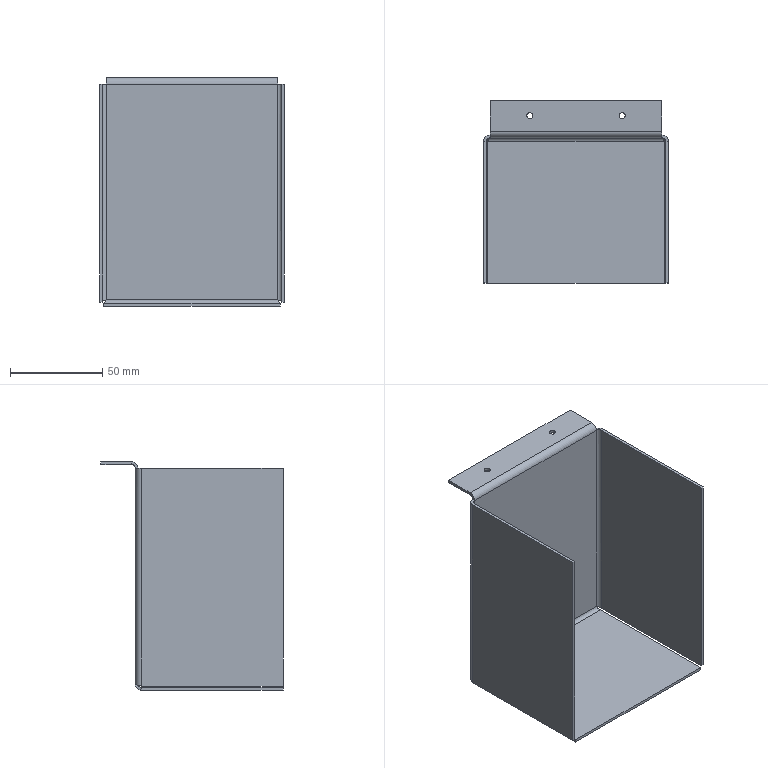Part | NX | features BREP 1 | 1 solid | 42 faces | box 100 x 98.5 x 123.5 mm | volume 59261 mm3 | plane 26 | cylinder 12 | spline 4 | commonest cylinder face diameters 3.3 x4 4 x4 7 x4
STEP:
#1=CARTESIAN_POINT('',(-26.65,10.5,63.5));
#2=VERTEX_POINT('',#1);
#3=CARTESIAN_POINT('',(-26.65,10.5,62.));
#4=VERTEX_POINT('',#3);
#5=CARTESIAN_POINT('',(-26.65,10.5,63.5));
#6=DIRECTION('',(0.,0.,1.));
#7=VECTOR('',#6,1000.);
#8=LINE('',#5,#7);
#9=EDGE_CURVE('',#2,#4,#8,.F.);
#10=ORIENTED_EDGE('',*,*,#9,.T.);
#11=CARTESIAN_POINT('',(-23.35,10.5,62.));
#12=VERTEX_POINT('',#11);
#13=CARTESIAN_POINT('',(-25.,10.5,62.));
#14=DIRECTION('',(0.,0.,1.));
#15=DIRECTION('',(0.,-1.,0.));
#16=AXIS2_PLACEMENT_3D('',#13,#14,#15);
#17=CIRCLE('',#16,1.65);
#18=EDGE_CURVE('',#12,#4,#17,.T.);
#19=ORIENTED_EDGE('',*,*,#18,.F.);
#20=CARTESIAN_POINT('',(-23.35,10.5,63.5));
#21=VERTEX_POINT('',#20);
#22=CARTESIAN_POINT('',(-23.35,10.5,63.5));
#23=DIRECTION('',(0.,0.,1.));
#24=VECTOR('',#23,1000.);
#25=LINE('',#22,#24);
#26=EDGE_CURVE('',#21,#12,#25,.F.);
#27=ORIENTED_EDGE('',*,*,#26,.F.);
#28=CARTESIAN_POINT('',(-25.,10.5,63.5));
#29=DIRECTION('',(0.,0.,1.));
#30=DIRECTION('',(1.,0.,0.));
#31=AXIS2_PLACEMENT_3D('',#28,#29,#30);
#32=CIRCLE('',#31,1.65);
#33=EDGE_CURVE('',#21,#2,#32,.T.);
#34=ORIENTED_EDGE('',*,*,#33,.T.);
#35=EDGE_LOOP('',(#10,#19,#27,#34));
#36=FACE_BOUND('',#35,.T.);
#37=CARTESIAN_POINT('',(-25.,10.5,63.5));
#38=DIRECTION('',(0.,0.,1.));
#39=DIRECTION('',(1.,0.,0.));
#40=AXIS2_PLACEMENT_3D('',#37,#38,#39);
#41=CYLINDRICAL_SURFACE('',#40,1.65);
#42=ADVANCED_FACE('',(#36),#41,.F.);
#43=CARTESIAN_POINT('',(23.35,10.5,63.5));
#44=VERTEX_POINT('',#43);
#45=CARTESIAN_POINT('',(23.35,10.5,62.));
#46=VERTEX_POINT('',#45);
#47=CARTESIAN_POINT('',(23.35,10.5,63.5));
#48=DIRECTION('',(0.,0.,1.));
#49=VECTOR('',#48,1000.);
#50=LINE('',#47,#49);
#51=EDGE_CURVE('',#44,#46,#50,.F.);
#52=ORIENTED_EDGE('',*,*,#51,.T.);
#53=CARTESIAN_POINT('',(26.65,10.5,62.));
#54=VERTEX_POINT('',#53);
#55=CARTESIAN_POINT('',(25.,10.5,62.));
#56=DIRECTION('',(0.,0.,1.));
#57=DIRECTION('',(0.,-1.,0.));
#58=AXIS2_PLACEMENT_3D('',#55,#56,#57);
#59=CIRCLE('',#58,1.65);
#60=EDGE_CURVE('',#54,#46,#59,.T.);
#61=ORIENTED_EDGE('',*,*,#60,.F.);
#62=CARTESIAN_POINT('',(26.65,10.5,63.5));
#63=VERTEX_POINT('',#62);
#64=CARTESIAN_POINT('',(26.65,10.5,63.5));
#65=DIRECTION('',(0.,0.,1.));
#66=VECTOR('',#65,1000.);
#67=LINE('',#64,#66);
#68=EDGE_CURVE('',#63,#54,#67,.F.);
#69=ORIENTED_EDGE('',*,*,#68,.F.);
#70=CARTESIAN_POINT('',(25.,10.5,63.5));
#71=DIRECTION('',(0.,0.,1.));
#72=DIRECTION('',(1.,0.,0.));
#73=AXIS2_PLACEMENT_3D('',#70,#71,#72);
#74=CIRCLE('',#73,1.65);
#75=EDGE_CURVE('',#63,#44,#74,.T.);
#76=ORIENTED_EDGE('',*,*,#75,.T.);
#77=EDGE_LOOP('',(#52,#61,#69,#76));
#78=FACE_BOUND('',#77,.T.);
#79=CARTESIAN_POINT('',(25.,10.5,63.5));
#80=DIRECTION('',(0.,0.,1.));
#81=DIRECTION('',(1.,0.,0.));
#82=AXIS2_PLACEMENT_3D('',#79,#80,#81);
#83=CYLINDRICAL_SURFACE('',#82,1.65);
#84=ADVANCED_FACE('',(#78),#83,.F.);
#85=CARTESIAN_POINT('',(-46.5,18.5,62.));
#86=VERTEX_POINT('',#85);
#87=CARTESIAN_POINT('',(46.5,18.5,62.));
#88=VERTEX_POINT('',#87);
#89=CARTESIAN_POINT('',(0.,18.5,62.));
#90=DIRECTION('',(1.,0.,0.));
#91=VECTOR('',#90,1000.);
#92=LINE('',#89,#91);
#93=EDGE_CURVE('',#86,#88,#92,.T.);
#94=ORIENTED_EDGE('',*,*,#93,.F.);
#95=CARTESIAN_POINT('',(-46.5,18.5,63.5));
#96=VERTEX_POINT('',#95);
#97=CARTESIAN_POINT('',(-46.5,18.5,63.5));
#98=DIRECTION('',(0.,0.,-1.));
#99=VECTOR('',#98,1000.);
#100=LINE('',#97,#99);
#101=EDGE_CURVE('',#96,#86,#100,.T.);
#102=ORIENTED_EDGE('',*,*,#101,.F.);
#103=CARTESIAN_POINT('',(46.5,18.5,63.5));
#104=VERTEX_POINT('',#103);
#105=CARTESIAN_POINT('',(46.5,18.5,63.5));
#106=DIRECTION('',(1.,0.,0.));
#107=VECTOR('',#106,1000.);
#108=LINE('',#105,#107);
#109=EDGE_CURVE('',#96,#104,#108,.T.);
#110=ORIENTED_EDGE('',*,*,#109,.T.);
#111=CARTESIAN_POINT('',(46.5,18.5,63.5));
#112=DIRECTION('',(0.,0.,-1.));
#113=VECTOR('',#112,1000.);
#114=LINE('',#111,#113);
#115=EDGE_CURVE('',#104,#88,#114,.T.);
#116=ORIENTED_EDGE('',*,*,#115,.T.);
#117=EDGE_LOOP('',(#94,#102,#110,#116));
#118=FACE_BOUND('',#117,.T.);
#119=CARTESIAN_POINT('',(46.5,18.5,63.5));
#120=DIRECTION('',(0.,1.,0.));
#121=DIRECTION('',(0.,0.,1.));
#122=AXIS2_PLACEMENT_3D('',#119,#120,#121);
#123=PLANE('',#122);
#124=ADVANCED_FACE('',(#118),#123,.T.);
#125=CARTESIAN_POINT('',(-46.5,2.,62.));
#126=VERTEX_POINT('',#125);
#127=CARTESIAN_POINT('',(46.5,2.,62.));
#128=VERTEX_POINT('',#127);
#129=CARTESIAN_POINT('',(-46.5,2.,62.));
#130=DIRECTION('',(1.,0.,0.));
#131=VECTOR('',#130,1000.);
#132=LINE('',#129,#131);
#133=EDGE_CURVE('',#126,#128,#132,.T.);
#134=ORIENTED_EDGE('',*,*,#133,.F.);
#135=CARTESIAN_POINT('',(-46.5,0.,62.));
#136=DIRECTION('',(0.,1.,0.));
#137=VECTOR('',#136,1000.);
#138=LINE('',#135,#137);
#139=EDGE_CURVE('',#126,#86,#138,.T.);
#140=ORIENTED_EDGE('',*,*,#139,.T.);
#141=ORIENTED_EDGE('',*,*,#93,.T.);
#142=CARTESIAN_POINT('',(46.5,0.,62.));
#143=DIRECTION('',(0.,-1.,0.));
#144=VECTOR('',#143,1000.);
#145=LINE('',#142,#144);
#146=EDGE_CURVE('',#88,#128,#145,.T.);
#147=ORIENTED_EDGE('',*,*,#146,.T.);
#148=EDGE_LOOP('',(#134,#140,#141,#147));
#149=FACE_BOUND('',#148,.T.);
#150=ORIENTED_EDGE('',*,*,#60,.T.);
#151=CARTESIAN_POINT('',(25.,10.5,62.));
#152=DIRECTION('',(0.,0.,1.));
#153=DIRECTION('',(0.,-1.,0.));
#154=AXIS2_PLACEMENT_3D('',#151,#152,#153);
#155=CIRCLE('',#154,1.65);
#156=EDGE_CURVE('',#46,#54,#155,.T.);
#157=ORIENTED_EDGE('',*,*,#156,.T.);
#158=EDGE_LOOP('',(#150,#157));
#159=FACE_BOUND('',#158,.T.);
#160=ORIENTED_EDGE('',*,*,#18,.T.);
#161=CARTESIAN_POINT('',(-25.,10.5,62.));
#162=DIRECTION('',(0.,0.,1.));
#163=DIRECTION('',(0.,-1.,0.));
#164=AXIS2_PLACEMENT_3D('',#161,#162,#163);
#165=CIRCLE('',#164,1.65);
#166=EDGE_CURVE('',#4,#12,#165,.T.);
#167=ORIENTED_EDGE('',*,*,#166,.T.);
#168=EDGE_LOOP('',(#160,#167));
#169=FACE_BOUND('',#168,.T.);
#170=CARTESIAN_POINT('',(0.,0.,62.));
#171=DIRECTION('',(0.,0.,1.));
#172=DIRECTION('',(0.,-1.,0.));
#173=AXIS2_PLACEMENT_3D('',#170,#171,#172);
#174=PLANE('',#173);
#175=ADVANCED_FACE('',(#149,#159,#169),#174,.F.);
#176=CARTESIAN_POINT('',(-46.5,2.,63.5));
#177=VERTEX_POINT('',#176);
#178=CARTESIAN_POINT('',(-46.5,18.5,63.5));
#179=DIRECTION('',(0.,1.,0.));
#180=VECTOR('',#179,1000.);
#181=LINE('',#178,#180);
#182=EDGE_CURVE('',#177,#96,#181,.T.);
#183=ORIENTED_EDGE('',*,*,#182,.F.);
#184=CARTESIAN_POINT('',(46.5,2.,63.5));
#185=VERTEX_POINT('',#184);
#186=CARTESIAN_POINT('',(0.,2.,63.5));
#187=DIRECTION('',(1.,0.,0.));
#188=VECTOR('',#187,1000.);
#189=LINE('',#186,#188);
#190=EDGE_CURVE('',#177,#185,#189,.T.);
#191=ORIENTED_EDGE('',*,*,#190,.T.);
#192=CARTESIAN_POINT('',(46.5,0.,63.5));
#193=DIRECTION('',(0.,-1.,0.));
#194=VECTOR('',#193,1000.);
#195=LINE('',#192,#194);
#196=EDGE_CURVE('',#104,#185,#195,.T.);
#197=ORIENTED_EDGE('',*,*,#196,.F.);
#198=ORIENTED_EDGE('',*,*,#109,.F.);
#199=EDGE_LOOP('',(#183,#191,#197,#198));
#200=FACE_BOUND('',#199,.T.);
#201=ORIENTED_EDGE('',*,*,#75,.F.);
#202=CARTESIAN_POINT('',(25.,10.5,63.5));
#203=DIRECTION('',(0.,0.,1.));
#204=DIRECTION('',(1.,0.,0.));
#205=AXIS2_PLACEMENT_3D('',#202,#203,#204);
#206=CIRCLE('',#205,1.65);
#207=EDGE_CURVE('',#44,#63,#206,.T.);
#208=ORIENTED_EDGE('',*,*,#207,.F.);
#209=EDGE_LOOP('',(#201,#208));
#210=FACE_BOUND('',#209,.T.);
#211=ORIENTED_EDGE('',*,*,#33,.F.);
#212=CARTESIAN_POINT('',(-25.,10.5,63.5));
#213=DIRECTION('',(0.,0.,1.));
#214=DIRECTION('',(1.,0.,0.));
#215=AXIS2_PLACEMENT_3D('',#212,#213,#214);
#216=CIRCLE('',#215,1.65);
#217=EDGE_CURVE('',#2,#21,#216,.T.);
#218=ORIENTED_EDGE('',*,*,#217,.F.);
#219=EDGE_LOOP('',(#211,#218));
#220=FACE_BOUND('',#219,.T.);
#221=CARTESIAN_POINT('',(0.,0.,63.5));
#222=DIRECTION('',(0.,0.,1.));
#223=DIRECTION('',(0.,-1.,0.));
#224=AXIS2_PLACEMENT_3D('',#221,#222,#223);
#225=PLANE('',#224);
#226=ADVANCED_FACE('',(#200,#210,#220),#225,.T.);
#227=ORIENTED_EDGE('',*,*,#139,.F.);
#228=CARTESIAN_POINT('',(-46.5,2.,63.5));
#229=DIRECTION('',(0.,0.,1.));
#230=VECTOR('',#229,1000.);
#231=LINE('',#228,#230);
#232=EDGE_CURVE('',#126,#177,#231,.T.);
#233=ORIENTED_EDGE('',*,*,#232,.T.);
#234=ORIENTED_EDGE('',*,*,#182,.T.);
#235=ORIENTED_EDGE('',*,*,#101,.T.);
#236=EDGE_LOOP('',(#227,#233,#234,#235));
#237=FACE_BOUND('',#236,.T.);
#238=CARTESIAN_POINT('',(-46.5,18.5,63.5));
#239=DIRECTION('',(-1.,0.,0.));
#240=DIRECTION('',(0.,-1.,0.));
#241=AXIS2_PLACEMENT_3D('',#238,#239,#240);
#242=PLANE('',#241);
#243=ADVANCED_FACE('',(#237),#242,.T.);
#244=ORIENTED_EDGE('',*,*,#196,.T.);
#245=CARTESIAN_POINT('',(46.5,2.,62.));
#246=DIRECTION('',(0.,0.,1.));
#247=VECTOR('',#246,1000.);
#248=LINE('',#245,#247);
#249=EDGE_CURVE('',#128,#185,#248,.T.);
#250=ORIENTED_EDGE('',*,*,#249,.F.);
#251=ORIENTED_EDGE('',*,*,#146,.F.);
#252=ORIENTED_EDGE('',*,*,#115,.F.);
#253=EDGE_LOOP('',(#244,#250,#251,#252));
#254=FACE_BOUND('',#253,.T.);
#255=CARTESIAN_POINT('',(46.5,0.,63.5));
#256=DIRECTION('',(1.,0.,0.));
#257=DIRECTION('',(0.,0.,-1.));
#258=AXIS2_PLACEMENT_3D('',#255,#256,#257);
#259=PLANE('',#258);
#260=ADVANCED_FACE('',(#254),#259,.T.);
#261=CARTESIAN_POINT('',(-46.5,0.,60.));
#262=VERTEX_POINT('',#261);
#263=CARTESIAN_POINT('',(46.5,0.,60.));
#264=VERTEX_POINT('',#263);
#265=CARTESIAN_POINT('',(50.,0.,60.));
#266=DIRECTION('',(1.,0.,0.));
#267=VECTOR('',#266,1000.);
#268=LINE('',#265,#267);
#269=EDGE_CURVE('',#262,#264,#268,.T.);
#270=ORIENTED_EDGE('',*,*,#269,.F.);
#271=CARTESIAN_POINT('',(-46.5,2.,60.));
#272=DIRECTION('',(-1.,0.,0.));
#273=DIRECTION('',(0.,0.,-1.));
#274=AXIS2_PLACEMENT_3D('',#271,#272,#273);
#275=CIRCLE('',#274,2.);
#276=EDGE_CURVE('',#262,#126,#275,.T.);
#277=ORIENTED_EDGE('',*,*,#276,.T.);
#278=ORIENTED_EDGE('',*,*,#133,.T.);
#279=CARTESIAN_POINT('',(46.5,2.,60.));
#280=DIRECTION('',(1.,0.,0.));
#281=DIRECTION('',(0.,0.,-1.));
#282=AXIS2_PLACEMENT_3D('',#279,#280,#281);
#283=CIRCLE('',#282,2.);
#284=EDGE_CURVE('',#128,#264,#283,.T.);
#285=ORIENTED_EDGE('',*,*,#284,.T.);
#286=EDGE_LOOP('',(#270,#277,#278,#285));
#287=FACE_BOUND('',#286,.T.);
#288=CARTESIAN_POINT('',(46.5,2.,60.));
#289=DIRECTION('',(1.,0.,0.));
#290=DIRECTION('',(0.,0.,1.));
#291=AXIS2_PLACEMENT_3D('',#288,#289,#290);
#292=CYLINDRICAL_SURFACE('',#291,2.);
#293=ADVANCED_FACE('',(#287),#292,.F.);
#294=CARTESIAN_POINT('',(-46.5,-1.5,60.));
#295=VERTEX_POINT('',#294);
#296=CARTESIAN_POINT('',(46.5,-1.5,60.));
#297=VERTEX_POINT('',#296);
#298=CARTESIAN_POINT('',(50.,-1.5,60.));
#299=DIRECTION('',(1.,0.,0.));
#300=VECTOR('',#299,1000.);
#301=LINE('',#298,#300);
#302=EDGE_CURVE('',#295,#297,#301,.T.);
#303=ORIENTED_EDGE('',*,*,#302,.T.);
#304=CARTESIAN_POINT('',(46.5,2.,60.));
#305=DIRECTION('',(1.,0.,0.));
#306=DIRECTION('',(0.,0.,-1.));
#307=AXIS2_PLACEMENT_3D('',#304,#305,#306);
#308=CIRCLE('',#307,3.5);
#309=EDGE_CURVE('',#185,#297,#308,.T.);
#310=ORIENTED_EDGE('',*,*,#309,.F.);
#311=ORIENTED_EDGE('',*,*,#190,.F.);
#312=CARTESIAN_POINT('',(-46.5,2.,60.));
#313=DIRECTION('',(-1.,0.,0.));
#314=DIRECTION('',(0.,0.,-1.));
#315=AXIS2_PLACEMENT_3D('',#312,#313,#314);
#316=CIRCLE('',#315,3.5);
#317=EDGE_CURVE('',#295,#177,#316,.T.);
#318=ORIENTED_EDGE('',*,*,#317,.F.);
#319=EDGE_LOOP('',(#303,#310,#311,#318));
#320=FACE_BOUND('',#319,.T.);
#321=CARTESIAN_POINT('',(46.5,2.,60.));
#322=DIRECTION('',(1.,0.,0.));
#323=DIRECTION('',(0.,0.,1.));
#324=AXIS2_PLACEMENT_3D('',#321,#322,#323);
#325=CYLINDRICAL_SURFACE('',#324,3.5);
#326=ADVANCED_FACE('',(#320),#325,.T.);
#327=ORIENTED_EDGE('',*,*,#284,.F.);
#328=ORIENTED_EDGE('',*,*,#249,.T.);
#329=ORIENTED_EDGE('',*,*,#309,.T.);
#330=CARTESIAN_POINT('',(46.5,-1.5,60.));
#331=DIRECTION('',(0.,1.,0.));
#332=VECTOR('',#331,1000.);
#333=LINE('',#330,#332);
#334=EDGE_CURVE('',#297,#264,#333,.T.);
#335=ORIENTED_EDGE('',*,*,#334,.T.);
#336=EDGE_LOOP('',(#327,#328,#329,#335));
#337=FACE_BOUND('',#336,.T.);
#338=CARTESIAN_POINT('',(46.5,2.,60.));
#339=DIRECTION('',(-1.,0.,0.));
#340=DIRECTION('',(0.,0.,1.));
#341=AXIS2_PLACEMENT_3D('',#338,#339,#340);
#342=PLANE('',#341);
#343=ADVANCED_FACE('',(#337),#342,.F.);
#344=ORIENTED_EDGE('',*,*,#232,.F.);
#345=ORIENTED_EDGE('',*,*,#276,.F.);
#346=CARTESIAN_POINT('',(-46.5,-1.5,60.));
#347=DIRECTION('',(0.,1.,0.));
#348=VECTOR('',#347,1000.);
#349=LINE('',#346,#348);
#350=EDGE_CURVE('',#295,#262,#349,.T.);
#351=ORIENTED_EDGE('',*,*,#350,.F.);
#352=ORIENTED_EDGE('',*,*,#317,.T.);
#353=EDGE_LOOP('',(#344,#345,#351,#352));
#354=FACE_BOUND('',#353,.T.);
#355=CARTESIAN_POINT('',(-46.5,2.,60.));
#356=DIRECTION('',(-1.,0.,0.));
#357=DIRECTION('',(0.,0.,1.));
#358=AXIS2_PLACEMENT_3D('',#355,#356,#357);
#359=PLANE('',#358);
#360=ADVANCED_FACE('',(#354),#359,.T.);
#361=CARTESIAN_POINT('',(47.793,-3.5,-58.5));
#362=VERTEX_POINT('',#361);
#363=CARTESIAN_POINT('',(47.793,-80.,-58.5));
#364=VERTEX_POINT('',#363);
#365=CARTESIAN_POINT('',(47.793,-1.5,-58.5));
#366=DIRECTION('',(0.,-1.,0.));
#367=VECTOR('',#366,1000.);
#368=LINE('',#365,#367);
#369=EDGE_CURVE('',#362,#364,#368,.T.);
#370=ORIENTED_EDGE('',*,*,#369,.T.);
#371=CARTESIAN_POINT('',(47.793,-80.,-60.));
#372=VERTEX_POINT('',#371);
#373=CARTESIAN_POINT('',(47.793,-80.,-58.5));
#374=DIRECTION('',(0.,0.,-1.));
#375=VECTOR('',#374,1000.);
#376=LINE('',#373,#375);
#377=EDGE_CURVE('',#364,#372,#376,.T.);
#378=ORIENTED_EDGE('',*,*,#377,.T.);
#379=CARTESIAN_POINT('',(47.793,-3.5,-60.));
#380=VERTEX_POINT('',#379);
#381=CARTESIAN_POINT('',(47.793,0.,-60.));
#382=DIRECTION('',(0.,-1.,0.));
#383=VECTOR('',#382,1000.);
#384=LINE('',#381,#383);
#385=EDGE_CURVE('',#380,#372,#384,.T.);
#386=ORIENTED_EDGE('',*,*,#385,.F.);
#387=CARTESIAN_POINT('',(47.793,-3.5,-58.5));
#388=DIRECTION('',(0.,0.,1.));
#389=VECTOR('',#388,1000.);
#390=LINE('',#387,#389);
#391=EDGE_CURVE('',#380,#362,#390,.T.);
#392=ORIENTED_EDGE('',*,*,#391,.T.);
#393=EDGE_LOOP('',(#370,#378,#386,#392));
#394=FACE_BOUND('',#393,.T.);
#395=CARTESIAN_POINT('',(47.793,-1.5,-58.5));
#396=DIRECTION('',(-1.,0.,0.));
#397=DIRECTION('',(0.,-1.,0.));
#398=AXIS2_PLACEMENT_3D('',#395,#396,#397);
#399=PLANE('',#398);
#400=ADVANCED_FACE('',(#394),#399,.F.);
#401=ORIENTED_EDGE('',*,*,#377,.F.);
#402=CARTESIAN_POINT('',(-47.793,-80.,-58.5));
#403=VERTEX_POINT('',#402);
#404=CARTESIAN_POINT('',(0.,-80.,-58.5));
#405=DIRECTION('',(1.,0.,0.));
#406=VECTOR('',#405,1000.);
#407=LINE('',#404,#406);
#408=EDGE_CURVE('',#403,#364,#407,.T.);
#409=ORIENTED_EDGE('',*,*,#408,.F.);
#410=CARTESIAN_POINT('',(-47.793,-80.,-60.));
#411=VERTEX_POINT('',#410);
#412=CARTESIAN_POINT('',(-47.793,-80.,-60.));
#413=DIRECTION('',(0.,0.,-1.));
#414=VECTOR('',#413,1000.);
#415=LINE('',#412,#414);
#416=EDGE_CURVE('',#403,#411,#415,.T.);
#417=ORIENTED_EDGE('',*,*,#416,.T.);
#418=CARTESIAN_POINT('',(-50.,-80.,-60.));
#419=DIRECTION('',(1.,0.,0.));
#420=VECTOR('',#419,1000.);
#421=LINE('',#418,#420);
#422=EDGE_CURVE('',#411,#372,#421,.T.);
#423=ORIENTED_EDGE('',*,*,#422,.T.);
#424=EDGE_LOOP('',(#401,#409,#417,#423));
#425=FACE_BOUND('',#424,.T.);
#426=CARTESIAN_POINT('',(-50.,-80.,-60.));
#427=DIRECTION('',(0.,-1.,0.));
#428=DIRECTION('',(0.,0.,-1.));
#429=AXIS2_PLACEMENT_3D('',#426,#427,#428);
#430=PLANE('',#429);
#431=ADVANCED_FACE('',(#425),#430,.T.);
#432=ORIENTED_EDGE('',*,*,#369,.F.);
#433=CARTESIAN_POINT('',(-47.793,-3.5,-58.5));
#434=VERTEX_POINT('',#433);
#435=CARTESIAN_POINT('',(-50.,-3.5,-58.5));
#436=DIRECTION('',(1.,0.,0.));
#437=VECTOR('',#436,1000.);
#438=LINE('',#435,#437);
#439=EDGE_CURVE('',#434,#362,#438,.T.);
#440=ORIENTED_EDGE('',*,*,#439,.F.);
#441=CARTESIAN_POINT('',(-47.793,0.,-58.5));
#442=DIRECTION('',(0.,-1.,0.));
#443=VECTOR('',#442,1000.);
#444=LINE('',#441,#443);
#445=EDGE_CURVE('',#434,#403,#444,.T.);
#446=ORIENTED_EDGE('',*,*,#445,.T.);
#447=ORIENTED_EDGE('',*,*,#408,.T.);
#448=EDGE_LOOP('',(#432,#440,#446,#447));
#449=FACE_BOUND('',#448,.T.);
#450=CARTESIAN_POINT('',(0.,0.,-58.5));
#451=DIRECTION('',(0.,0.,1.));
#452=DIRECTION('',(0.,-1.,0.));
#453=AXIS2_PLACEMENT_3D('',#450,#451,#452);
#454=PLANE('',#453);
#455=ADVANCED_FACE('',(#449),#454,.T.);
#456=CARTESIAN_POINT('',(-47.793,-3.5,-60.));
#457=VERTEX_POINT('',#456);
#458=CARTESIAN_POINT('',(-50.,-3.5,-60.));
#459=DIRECTION('',(-1.,0.,0.));
#460=VECTOR('',#459,1000.);
#461=LINE('',#458,#460);
#462=EDGE_CURVE('',#380,#457,#461,.T.);
#463=ORIENTED_EDGE('',*,*,#462,.F.);
#464=ORIENTED_EDGE('',*,*,#385,.T.);
#465=ORIENTED_EDGE('',*,*,#422,.F.);
#466=CARTESIAN_POINT('',(-47.793,-1.5,-60.));
#467=DIRECTION('',(0.,-1.,0.));
#468=VECTOR('',#467,1000.);
#469=LINE('',#466,#468);
#470=EDGE_CURVE('',#457,#411,#469,.T.);
#471=ORIENTED_EDGE('',*,*,#470,.F.);
#472=EDGE_LOOP('',(#463,#464,#465,#471));
#473=FACE_BOUND('',#472,.T.);
#474=CARTESIAN_POINT('',(0.,0.,-60.));
#475=DIRECTION('',(0.,0.,1.));
#476=DIRECTION('',(0.,-1.,0.));
#477=AXIS2_PLACEMENT_3D('',#474,#475,#476);
#478=PLANE('',#477);
#479=ADVANCED_FACE('',(#473),#478,.F.);
#480=ORIENTED_EDGE('',*,*,#416,.F.);
#481=ORIENTED_EDGE('',*,*,#445,.F.);
#482=CARTESIAN_POINT('',(-47.793,-3.5,-58.5));
#483=DIRECTION('',(0.,0.,1.));
#484=VECTOR('',#483,1000.);
#485=LINE('',#482,#484);
#486=EDGE_CURVE('',#457,#434,#485,.T.);
#487=ORIENTED_EDGE('',*,*,#486,.F.);
#488=ORIENTED_EDGE('',*,*,#470,.T.);
#489=EDGE_LOOP('',(#480,#481,#487,#488));
#490=FACE_BOUND('',#489,.T.);
#491=CARTESIAN_POINT('',(-47.793,-1.5,-58.5));
#492=DIRECTION('',(-1.,0.,0.));
#493=DIRECTION('',(0.,-1.,0.));
#494=AXIS2_PLACEMENT_3D('',#491,#492,#493);
#495=PLANE('',#494);
#496=ADVANCED_FACE('',(#490),#495,.T.);
#497=CARTESIAN_POINT('',(46.5,-1.5,-56.5));
#498=VERTEX_POINT('',#497);
#499=CARTESIAN_POINT('',(-46.5,-1.5,-56.5));
#500=VERTEX_POINT('',#499);
#501=CARTESIAN_POINT('',(47.793,-1.5,-56.5));
#502=DIRECTION('',(-1.,0.,0.));
#503=VECTOR('',#502,1000.);
#504=LINE('',#501,#503);
#505=EDGE_CURVE('',#498,#500,#504,.T.);
#506=ORIENTED_EDGE('',*,*,#505,.T.);
#507=CARTESIAN_POINT('',(-46.5,-1.5,-56.5));
#508=CARTESIAN_POINT('',(-46.715,-1.5,-57.024));
#509=CARTESIAN_POINT('',(-47.146,-1.933,-58.067));
#510=CARTESIAN_POINT('',(-47.577,-2.976,-58.5));
#511=CARTESIAN_POINT('',(-47.793,-3.5,-58.5));
#512=B_SPLINE_CURVE_WITH_KNOTS('',3,(#507,#508,#509,#510,#511),.UNSPECIFIED.,.F.,.F.,(4,1,4),(0.,0.5,1.),.UNSPECIFIED.);
#513=EDGE_CURVE('',#500,#434,#512,.T.);
#514=ORIENTED_EDGE('',*,*,#513,.T.);
#515=ORIENTED_EDGE('',*,*,#439,.T.);
#516=CARTESIAN_POINT('',(47.793,-3.5,-58.5));
#517=CARTESIAN_POINT('',(47.577,-2.976,-58.5));
#518=CARTESIAN_POINT('',(47.146,-1.933,-58.067));
#519=CARTESIAN_POINT('',(46.715,-1.5,-57.024));
#520=CARTESIAN_POINT('',(46.5,-1.5,-56.5));
#521=B_SPLINE_CURVE_WITH_KNOTS('',3,(#516,#517,#518,#519,#520),.UNSPECIFIED.,.F.,.F.,(4,1,4),(0.,0.5,1.),.UNSPECIFIED.);
#522=EDGE_CURVE('',#362,#498,#521,.T.);
#523=ORIENTED_EDGE('',*,*,#522,.T.);
#524=EDGE_LOOP('',(#506,#514,#515,#523));
#525=FACE_BOUND('',#524,.T.);
#526=CARTESIAN_POINT('',(47.793,-3.5,-56.5));
#527=DIRECTION('',(1.,0.,0.));
#528=DIRECTION('',(0.,0.,-1.));
#529=AXIS2_PLACEMENT_3D('',#526,#527,#528);
#530=CYLINDRICAL_SURFACE('',#529,2.);
#531=ADVANCED_FACE('',(#525),#530,.F.);
#532=CARTESIAN_POINT('',(46.5,0.,-56.5));
#533=VERTEX_POINT('',#532);
#534=CARTESIAN_POINT('',(-46.5,0.,-56.5));
#535=VERTEX_POINT('',#534);
#536=CARTESIAN_POINT('',(47.793,0.,-56.5));
#537=DIRECTION('',(-1.,0.,0.));
#538=VECTOR('',#537,1000.);
#539=LINE('',#536,#538);
#540=EDGE_CURVE('',#533,#535,#539,.T.);
#541=ORIENTED_EDGE('',*,*,#540,.F.);
#542=CARTESIAN_POINT('',(46.5,0.,-56.5));
#543=CARTESIAN_POINT('',(46.715,0.,-57.416));
#544=CARTESIAN_POINT('',(47.146,-0.7584,-59.242));
#545=CARTESIAN_POINT('',(47.577,-2.584,-60.));
#546=CARTESIAN_POINT('',(47.793,-3.5,-60.));
#547=B_SPLINE_CURVE_WITH_KNOTS('',3,(#542,#543,#544,#545,#546),.UNSPECIFIED.,.F.,.F.,(4,1,4),(0.,0.5,1.),.UNSPECIFIED.);
#548=EDGE_CURVE('',#380,#533,#547,.F.);
#549=ORIENTED_EDGE('',*,*,#548,.F.);
#550=ORIENTED_EDGE('',*,*,#462,.T.);
#551=CARTESIAN_POINT('',(-47.793,-3.5,-60.));
#552=CARTESIAN_POINT('',(-47.577,-2.584,-60.));
#553=CARTESIAN_POINT('',(-47.146,-0.7584,-59.242));
#554=CARTESIAN_POINT('',(-46.715,0.,-57.416));
#555=CARTESIAN_POINT('',(-46.5,0.,-56.5));
#556=B_SPLINE_CURVE_WITH_KNOTS('',3,(#551,#552,#553,#554,#555),.UNSPECIFIED.,.F.,.F.,(4,1,4),(0.,0.5,1.),.UNSPECIFIED.);
#557=EDGE_CURVE('',#535,#457,#556,.F.);
#558=ORIENTED_EDGE('',*,*,#557,.F.);
#559=EDGE_LOOP('',(#541,#549,#550,#558));
#560=FACE_BOUND('',#559,.T.);
#561=CARTESIAN_POINT('',(47.793,-3.5,-56.5));
#562=DIRECTION('',(1.,0.,0.));
#563=DIRECTION('',(0.,0.,-1.));
#564=AXIS2_PLACEMENT_3D('',#561,#562,#563);
#565=CYLINDRICAL_SURFACE('',#564,3.5);
#566=ADVANCED_FACE('',(#560),#565,.T.);
#567=ORIENTED_EDGE('',*,*,#522,.F.);
#568=ORIENTED_EDGE('',*,*,#391,.F.);
#569=ORIENTED_EDGE('',*,*,#548,.T.);
#570=CARTESIAN_POINT('',(46.5,-1.5,-56.5));
#571=DIRECTION('',(0.,1.,0.));
#572=VECTOR('',#571,1000.);
#573=LINE('',#570,#572);
#574=EDGE_CURVE('',#498,#533,#573,.T.);
#575=ORIENTED_EDGE('',*,*,#574,.F.);
#576=EDGE_LOOP('',(#567,#568,#569,#575));
#577=FACE_BOUND('',#576,.T.);
#578=CARTESIAN_POINT('',(47.793,-3.5,-60.015));
#579=CARTESIAN_POINT('',(47.685,-3.04,-60.015));
#580=CARTESIAN_POINT('',(47.577,-2.58,-59.924));
#581=CARTESIAN_POINT('',(47.362,-1.73,-59.571));
#582=CARTESIAN_POINT('',(47.254,-1.34,-59.311));
#583=CARTESIAN_POINT('',(47.039,-0.6892,-58.66));
#584=CARTESIAN_POINT('',(46.931,-0.4286,-58.27));
#585=CARTESIAN_POINT('',(46.715,-0.07649,-57.42));
#586=CARTESIAN_POINT('',(46.608,0.015,-56.96));
#587=CARTESIAN_POINT('',(46.5,0.015,-56.5));
#588=CARTESIAN_POINT('',(47.793,-3.5,-60.));
#589=CARTESIAN_POINT('',(47.685,-3.042,-60.));
#590=CARTESIAN_POINT('',(47.577,-2.584,-59.909));
#591=CARTESIAN_POINT('',(47.362,-1.737,-59.558));
#592=CARTESIAN_POINT('',(47.254,-1.349,-59.299));
#593=CARTESIAN_POINT('',(47.039,-0.7012,-58.651));
#594=CARTESIAN_POINT('',(46.931,-0.4417,-58.263));
#595=CARTESIAN_POINT('',(46.715,-0.0911,-57.416));
#596=CARTESIAN_POINT('',(46.608,0.,-56.958));
#597=CARTESIAN_POINT('',(46.5,0.,-56.5));
#598=CARTESIAN_POINT('',(47.793,-3.5,-58.5));
#599=CARTESIAN_POINT('',(47.685,-3.238,-58.5));
#600=CARTESIAN_POINT('',(47.577,-2.977,-58.448));
#601=CARTESIAN_POINT('',(47.362,-2.493,-58.248));
#602=CARTESIAN_POINT('',(47.254,-2.271,-58.099));
#603=CARTESIAN_POINT('',(47.039,-1.901,-57.729));
#604=CARTESIAN_POINT('',(46.931,-1.752,-57.507));
#605=CARTESIAN_POINT('',(46.715,-1.552,-57.023));
#606=CARTESIAN_POINT('',(46.608,-1.5,-56.762));
#607=CARTESIAN_POINT('',(46.5,-1.5,-56.5));
#608=CARTESIAN_POINT('',(47.793,-3.5,-58.485));
#609=CARTESIAN_POINT('',(47.685,-3.24,-58.485));
#610=CARTESIAN_POINT('',(47.577,-2.98,-58.433));
#611=CARTESIAN_POINT('',(47.362,-2.5,-58.234));
#612=CARTESIAN_POINT('',(47.254,-2.28,-58.087));
#613=CARTESIAN_POINT('',(47.039,-1.913,-57.72));
#614=CARTESIAN_POINT('',(46.931,-1.766,-57.5));
#615=CARTESIAN_POINT('',(46.715,-1.567,-57.02));
#616=CARTESIAN_POINT('',(46.608,-1.515,-56.76));
#617=CARTESIAN_POINT('',(46.5,-1.515,-56.5));
#618=B_SPLINE_SURFACE_WITH_KNOTS('',1,3,((#578,#579,#580,#581,#582,#583,#584,#585,#586,#587),(#588,#589,#590,#591,#592,#593,#594,#595,#596,#597),(#598,#599,#600,#601,#602,#603,#604,#605,#606,#607),(#608,#609,#610,#611,#612,#613,#614,#615,#616,#617)),.RULED_SURF.,.F.,.F.,.F.,(2,1,1,2),(4,2,2,2,4),(-0.01,0.,1.,1.01),(0.,0.25,0.5,0.75,1.),.UNSPECIFIED.);
#619=ADVANCED_FACE('',(#577),#618,.F.);
#620=ORIENTED_EDGE('',*,*,#486,.T.);
#621=ORIENTED_EDGE('',*,*,#513,.F.);
#622=CARTESIAN_POINT('',(-46.5,-1.5,-56.5));
#623=DIRECTION('',(0.,1.,0.));
#624=VECTOR('',#623,1000.);
#625=LINE('',#622,#624);
#626=EDGE_CURVE('',#500,#535,#625,.T.);
#627=ORIENTED_EDGE('',*,*,#626,.T.);
#628=ORIENTED_EDGE('',*,*,#557,.T.);
#629=EDGE_LOOP('',(#620,#621,#627,#628));
#630=FACE_BOUND('',#629,.T.);
#631=CARTESIAN_POINT('',(-46.5,0.015,-56.5));
#632=CARTESIAN_POINT('',(-46.608,0.015,-56.96));
#633=CARTESIAN_POINT('',(-46.715,-0.07649,-57.42));
#634=CARTESIAN_POINT('',(-46.931,-0.4286,-58.27));
#635=CARTESIAN_POINT('',(-47.039,-0.6892,-58.66));
#636=CARTESIAN_POINT('',(-47.254,-1.34,-59.311));
#637=CARTESIAN_POINT('',(-47.362,-1.73,-59.571));
#638=CARTESIAN_POINT('',(-47.577,-2.58,-59.924));
#639=CARTESIAN_POINT('',(-47.685,-3.04,-60.015));
#640=CARTESIAN_POINT('',(-47.793,-3.5,-60.015));
#641=CARTESIAN_POINT('',(-46.5,0.,-56.5));
#642=CARTESIAN_POINT('',(-46.608,0.,-56.958));
#643=CARTESIAN_POINT('',(-46.715,-0.0911,-57.416));
#644=CARTESIAN_POINT('',(-46.931,-0.4417,-58.263));
#645=CARTESIAN_POINT('',(-47.039,-0.7012,-58.651));
#646=CARTESIAN_POINT('',(-47.254,-1.349,-59.299));
#647=CARTESIAN_POINT('',(-47.362,-1.737,-59.558));
#648=CARTESIAN_POINT('',(-47.577,-2.584,-59.909));
#649=CARTESIAN_POINT('',(-47.685,-3.042,-60.));
#650=CARTESIAN_POINT('',(-47.793,-3.5,-60.));
#651=CARTESIAN_POINT('',(-46.5,-1.5,-56.5));
#652=CARTESIAN_POINT('',(-46.608,-1.5,-56.762));
#653=CARTESIAN_POINT('',(-46.715,-1.552,-57.023));
#654=CARTESIAN_POINT('',(-46.931,-1.752,-57.507));
#655=CARTESIAN_POINT('',(-47.039,-1.901,-57.729));
#656=CARTESIAN_POINT('',(-47.254,-2.271,-58.099));
#657=CARTESIAN_POINT('',(-47.362,-2.493,-58.248));
#658=CARTESIAN_POINT('',(-47.577,-2.977,-58.448));
#659=CARTESIAN_POINT('',(-47.685,-3.238,-58.5));
#660=CARTESIAN_POINT('',(-47.793,-3.5,-58.5));
#661=CARTESIAN_POINT('',(-46.5,-1.515,-56.5));
#662=CARTESIAN_POINT('',(-46.608,-1.515,-56.76));
#663=CARTESIAN_POINT('',(-46.715,-1.567,-57.02));
#664=CARTESIAN_POINT('',(-46.931,-1.766,-57.5));
#665=CARTESIAN_POINT('',(-47.039,-1.913,-57.72));
#666=CARTESIAN_POINT('',(-47.254,-2.28,-58.087));
#667=CARTESIAN_POINT('',(-47.362,-2.5,-58.234));
#668=CARTESIAN_POINT('',(-47.577,-2.98,-58.433));
#669=CARTESIAN_POINT('',(-47.685,-3.24,-58.485));
#670=CARTESIAN_POINT('',(-47.793,-3.5,-58.485));
#671=B_SPLINE_SURFACE_WITH_KNOTS('',1,3,((#631,#632,#633,#634,#635,#636,#637,#638,#639,#640),(#641,#642,#643,#644,#645,#646,#647,#648,#649,#650),(#651,#652,#653,#654,#655,#656,#657,#658,#659,#660),(#661,#662,#663,#664,#665,#666,#667,#668,#669,#670)),.RULED_SURF.,.F.,.F.,.F.,(2,1,1,2),(4,2,2,2,4),(-0.01,0.,1.,1.01),(0.,0.25,0.5,0.75,1.),.UNSPECIFIED.);
#672=ADVANCED_FACE('',(#630),#671,.F.);
#673=CARTESIAN_POINT('',(50.,-80.,60.));
#674=VERTEX_POINT('',#673);
#675=CARTESIAN_POINT('',(50.,-3.5,60.));
#676=VERTEX_POINT('',#675);
#677=CARTESIAN_POINT('',(50.,-80.,60.));
#678=DIRECTION('',(0.,1.,0.));
#679=VECTOR('',#678,1000.);
#680=LINE('',#677,#679);
#681=EDGE_CURVE('',#674,#676,#680,.T.);
#682=ORIENTED_EDGE('',*,*,#681,.T.);
#683=CARTESIAN_POINT('',(48.5,-3.5,60.));
#684=VERTEX_POINT('',#683);
#685=CARTESIAN_POINT('',(48.5,-3.5,60.));
#686=DIRECTION('',(1.,0.,0.));
#687=VECTOR('',#686,1000.);
#688=LINE('',#685,#687);
#689=EDGE_CURVE('',#684,#676,#688,.T.);
#690=ORIENTED_EDGE('',*,*,#689,.F.);
#691=CARTESIAN_POINT('',(48.5,-80.,60.));
#692=VERTEX_POINT('',#691);
#693=CARTESIAN_POINT('',(48.5,0.,60.));
#694=DIRECTION('',(0.,1.,0.));
#695=VECTOR('',#694,1000.);
#696=LINE('',#693,#695);
#697=EDGE_CURVE('',#692,#684,#696,.T.);
#698=ORIENTED_EDGE('',*,*,#697,.F.);
#699=CARTESIAN_POINT('',(50.,-80.,60.));
#700=DIRECTION('',(-1.,0.,0.));
#701=VECTOR('',#700,1000.);
#702=LINE('',#699,#701);
#703=EDGE_CURVE('',#674,#692,#702,.T.);
#704=ORIENTED_EDGE('',*,*,#703,.F.);
#705=EDGE_LOOP('',(#682,#690,#698,#704));
#706=FACE_BOUND('',#705,.T.);
#707=CARTESIAN_POINT('',(50.,-80.,60.));
#708=DIRECTION('',(0.,0.,1.));
#709=DIRECTION('',(0.,-1.,0.));
#710=AXIS2_PLACEMENT_3D('',#707,#708,#709);
#711=PLANE('',#710);
#712=ADVANCED_FACE('',(#706),#711,.T.);
#713=CARTESIAN_POINT('',(48.5,-80.,-57.793));
#714=VERTEX_POINT('',#713);
#715=CARTESIAN_POINT('',(48.5,-80.,0.));
#716=DIRECTION('',(0.,0.,1.));
#717=VECTOR('',#716,1000.);
#718=LINE('',#715,#717);
#719=EDGE_CURVE('',#714,#692,#718,.T.);
#720=ORIENTED_EDGE('',*,*,#719,.F.);
#721=CARTESIAN_POINT('',(50.,-80.,-57.793));
#722=VERTEX_POINT('',#721);
#723=CARTESIAN_POINT('',(50.,-80.,-57.793));
#724=DIRECTION('',(1.,0.,0.));
#725=VECTOR('',#724,1000.);
#726=LINE('',#723,#725);
#727=EDGE_CURVE('',#714,#722,#726,.T.);
#728=ORIENTED_EDGE('',*,*,#727,.T.);
#729=CARTESIAN_POINT('',(50.,-80.,-60.));
#730=DIRECTION('',(0.,0.,1.));
#731=VECTOR('',#730,1000.);
#732=LINE('',#729,#731);
#733=EDGE_CURVE('',#722,#674,#732,.T.);
#734=ORIENTED_EDGE('',*,*,#733,.T.);
#735=ORIENTED_EDGE('',*,*,#703,.T.);
#736=EDGE_LOOP('',(#720,#728,#734,#735));
#737=FACE_BOUND('',#736,.T.);
#738=CARTESIAN_POINT('',(50.,-80.,-60.));
#739=DIRECTION('',(0.,-1.,0.));
#740=DIRECTION('',(1.,0.,0.));
#741=AXIS2_PLACEMENT_3D('',#738,#739,#740);
#742=PLANE('',#741);
#743=ADVANCED_FACE('',(#737),#742,.T.);
#744=CARTESIAN_POINT('',(48.5,-3.5,-57.793));
#745=VERTEX_POINT('',#744);
#746=CARTESIAN_POINT('',(48.5,-3.5,-60.));
#747=DIRECTION('',(0.,0.,1.));
#748=VECTOR('',#747,1000.);
#749=LINE('',#746,#748);
#750=EDGE_CURVE('',#745,#684,#749,.T.);
#751=ORIENTED_EDGE('',*,*,#750,.F.);
#752=CARTESIAN_POINT('',(48.5,0.,-57.793));
#753=DIRECTION('',(0.,-1.,0.));
#754=VECTOR('',#753,1000.);
#755=LINE('',#752,#754);
#756=EDGE_CURVE('',#745,#714,#755,.T.);
#757=ORIENTED_EDGE('',*,*,#756,.T.);
#758=ORIENTED_EDGE('',*,*,#719,.T.);
#759=ORIENTED_EDGE('',*,*,#697,.T.);
#760=EDGE_LOOP('',(#751,#757,#758,#759));
#761=FACE_BOUND('',#760,.T.);
#762=CARTESIAN_POINT('',(48.5,0.,0.));
#763=DIRECTION('',(-1.,0.,0.));
#764=DIRECTION('',(0.,-1.,0.));
#765=AXIS2_PLACEMENT_3D('',#762,#763,#764);
#766=PLANE('',#765);
#767=ADVANCED_FACE('',(#761),#766,.T.);
#768=CARTESIAN_POINT('',(50.,-3.5,-57.793));
#769=VERTEX_POINT('',#768);
#770=CARTESIAN_POINT('',(50.,-1.5,-57.793));
#771=DIRECTION('',(0.,-1.,0.));
#772=VECTOR('',#771,1000.);
#773=LINE('',#770,#772);
#774=EDGE_CURVE('',#769,#722,#773,.T.);
#775=ORIENTED_EDGE('',*,*,#774,.F.);
#776=CARTESIAN_POINT('',(50.,-3.5,-60.));
#777=DIRECTION('',(0.,0.,-1.));
#778=VECTOR('',#777,1000.);
#779=LINE('',#776,#778);
#780=EDGE_CURVE('',#676,#769,#779,.T.);
#781=ORIENTED_EDGE('',*,*,#780,.F.);
#782=ORIENTED_EDGE('',*,*,#681,.F.);
#783=ORIENTED_EDGE('',*,*,#733,.F.);
#784=EDGE_LOOP('',(#775,#781,#782,#783));
#785=FACE_BOUND('',#784,.T.);
#786=CARTESIAN_POINT('',(50.,0.,0.));
#787=DIRECTION('',(-1.,0.,0.));
#788=DIRECTION('',(0.,-1.,0.));
#789=AXIS2_PLACEMENT_3D('',#786,#787,#788);
#790=PLANE('',#789);
#791=ADVANCED_FACE('',(#785),#790,.F.);
#792=ORIENTED_EDGE('',*,*,#727,.F.);
#793=ORIENTED_EDGE('',*,*,#756,.F.);
#794=CARTESIAN_POINT('',(48.5,-3.5,-57.793));
#795=DIRECTION('',(-1.,0.,0.));
#796=VECTOR('',#795,1000.);
#797=LINE('',#794,#796);
#798=EDGE_CURVE('',#769,#745,#797,.T.);
#799=ORIENTED_EDGE('',*,*,#798,.F.);
#800=ORIENTED_EDGE('',*,*,#774,.T.);
#801=EDGE_LOOP('',(#792,#793,#799,#800));
#802=FACE_BOUND('',#801,.T.);
#803=CARTESIAN_POINT('',(48.5,-1.5,-57.793));
#804=DIRECTION('',(0.,0.,-1.));
#805=DIRECTION('',(0.,1.,0.));
#806=AXIS2_PLACEMENT_3D('',#803,#804,#805);
#807=PLANE('',#806);
#808=ADVANCED_FACE('',(#802),#807,.T.);
#809=CARTESIAN_POINT('',(46.5,-1.5,60.));
#810=DIRECTION('',(0.,0.,-1.));
#811=VECTOR('',#810,1000.);
#812=LINE('',#809,#811);
#813=EDGE_CURVE('',#297,#498,#812,.T.);
#814=ORIENTED_EDGE('',*,*,#813,.T.);
#815=CARTESIAN_POINT('',(46.5,-1.5,-56.5));
#816=CARTESIAN_POINT('',(47.024,-1.5,-56.715));
#817=CARTESIAN_POINT('',(48.067,-1.933,-57.146));
#818=CARTESIAN_POINT('',(48.5,-2.976,-57.577));
#819=CARTESIAN_POINT('',(48.5,-3.5,-57.793));
#820=B_SPLINE_CURVE_WITH_KNOTS('',3,(#815,#816,#817,#818,#819),.UNSPECIFIED.,.F.,.F.,(4,1,4),(0.,0.5,1.),.UNSPECIFIED.);
#821=EDGE_CURVE('',#498,#745,#820,.T.);
#822=ORIENTED_EDGE('',*,*,#821,.T.);
#823=ORIENTED_EDGE('',*,*,#750,.T.);
#824=CARTESIAN_POINT('',(46.5,-3.5,60.));
#825=DIRECTION('',(0.,0.,1.));
#826=DIRECTION('',(1.,0.,0.));
#827=AXIS2_PLACEMENT_3D('',#824,#825,#826);
#828=CIRCLE('',#827,2.);
#829=EDGE_CURVE('',#684,#297,#828,.T.);
#830=ORIENTED_EDGE('',*,*,#829,.T.);
#831=EDGE_LOOP('',(#814,#822,#823,#830));
#832=FACE_BOUND('',#831,.T.);
#833=CARTESIAN_POINT('',(46.5,-3.5,60.));
#834=DIRECTION('',(0.,0.,1.));
#835=DIRECTION('',(1.,0.,0.));
#836=AXIS2_PLACEMENT_3D('',#833,#834,#835);
#837=CYLINDRICAL_SURFACE('',#836,2.);
#838=ADVANCED_FACE('',(#832),#837,.F.);
#839=CARTESIAN_POINT('',(46.5,0.,60.));
#840=DIRECTION('',(0.,0.,-1.));
#841=VECTOR('',#840,1000.);
#842=LINE('',#839,#841);
#843=EDGE_CURVE('',#264,#533,#842,.T.);
#844=ORIENTED_EDGE('',*,*,#843,.F.);
#845=CARTESIAN_POINT('',(46.5,-3.5,60.));
#846=DIRECTION('',(0.,0.,1.));
#847=DIRECTION('',(1.,0.,0.));
#848=AXIS2_PLACEMENT_3D('',#845,#846,#847);
#849=CIRCLE('',#848,3.5);
#850=EDGE_CURVE('',#676,#264,#849,.T.);
#851=ORIENTED_EDGE('',*,*,#850,.F.);
#852=ORIENTED_EDGE('',*,*,#780,.T.);
#853=CARTESIAN_POINT('',(50.,-3.5,-57.793));
#854=CARTESIAN_POINT('',(50.,-2.584,-57.577));
#855=CARTESIAN_POINT('',(49.242,-0.7584,-57.146));
#856=CARTESIAN_POINT('',(47.416,0.,-56.715));
#857=CARTESIAN_POINT('',(46.5,0.,-56.5));
#858=B_SPLINE_CURVE_WITH_KNOTS('',3,(#853,#854,#855,#856,#857),.UNSPECIFIED.,.F.,.F.,(4,1,4),(0.,0.5,1.),.UNSPECIFIED.);
#859=EDGE_CURVE('',#533,#769,#858,.F.);
#860=ORIENTED_EDGE('',*,*,#859,.F.);
#861=EDGE_LOOP('',(#844,#851,#852,#860));
#862=FACE_BOUND('',#861,.T.);
#863=CARTESIAN_POINT('',(46.5,-3.5,60.));
#864=DIRECTION('',(0.,0.,1.));
#865=DIRECTION('',(1.,0.,0.));
#866=AXIS2_PLACEMENT_3D('',#863,#864,#865);
#867=CYLINDRICAL_SURFACE('',#866,3.5);
#868=ADVANCED_FACE('',(#862),#867,.T.);
#869=ORIENTED_EDGE('',*,*,#829,.F.);
#870=ORIENTED_EDGE('',*,*,#689,.T.);
#871=ORIENTED_EDGE('',*,*,#850,.T.);
#872=ORIENTED_EDGE('',*,*,#334,.F.);
#873=EDGE_LOOP('',(#869,#870,#871,#872));
#874=FACE_BOUND('',#873,.T.);
#875=CARTESIAN_POINT('',(46.5,-3.5,60.));
#876=DIRECTION('',(0.,0.,-1.));
#877=DIRECTION('',(-1.,0.,0.));
#878=AXIS2_PLACEMENT_3D('',#875,#876,#877);
#879=PLANE('',#878);
#880=ADVANCED_FACE('',(#874),#879,.F.);
#881=ORIENTED_EDGE('',*,*,#798,.T.);
#882=ORIENTED_EDGE('',*,*,#821,.F.);
#883=ORIENTED_EDGE('',*,*,#574,.T.);
#884=ORIENTED_EDGE('',*,*,#859,.T.);
#885=EDGE_LOOP('',(#881,#882,#883,#884));
#886=FACE_BOUND('',#885,.T.);
#887=CARTESIAN_POINT('',(46.5,0.015,-56.5));
#888=CARTESIAN_POINT('',(46.96,0.015,-56.608));
#889=CARTESIAN_POINT('',(47.42,-0.07649,-56.715));
#890=CARTESIAN_POINT('',(48.27,-0.4286,-56.931));
#891=CARTESIAN_POINT('',(48.66,-0.6892,-57.039));
#892=CARTESIAN_POINT('',(49.311,-1.34,-57.254));
#893=CARTESIAN_POINT('',(49.571,-1.73,-57.362));
#894=CARTESIAN_POINT('',(49.924,-2.58,-57.577));
#895=CARTESIAN_POINT('',(50.015,-3.04,-57.685));
#896=CARTESIAN_POINT('',(50.015,-3.5,-57.793));
#897=CARTESIAN_POINT('',(46.5,0.,-56.5));
#898=CARTESIAN_POINT('',(46.958,0.,-56.608));
#899=CARTESIAN_POINT('',(47.416,-0.0911,-56.715));
#900=CARTESIAN_POINT('',(48.263,-0.4417,-56.931));
#901=CARTESIAN_POINT('',(48.651,-0.7012,-57.039));
#902=CARTESIAN_POINT('',(49.299,-1.349,-57.254));
#903=CARTESIAN_POINT('',(49.558,-1.737,-57.362));
#904=CARTESIAN_POINT('',(49.909,-2.584,-57.577));
#905=CARTESIAN_POINT('',(50.,-3.042,-57.685));
#906=CARTESIAN_POINT('',(50.,-3.5,-57.793));
#907=CARTESIAN_POINT('',(46.5,-1.5,-56.5));
#908=CARTESIAN_POINT('',(46.762,-1.5,-56.608));
#909=CARTESIAN_POINT('',(47.023,-1.552,-56.715));
#910=CARTESIAN_POINT('',(47.507,-1.752,-56.931));
#911=CARTESIAN_POINT('',(47.729,-1.901,-57.039));
#912=CARTESIAN_POINT('',(48.099,-2.271,-57.254));
#913=CARTESIAN_POINT('',(48.248,-2.493,-57.362));
#914=CARTESIAN_POINT('',(48.448,-2.977,-57.577));
#915=CARTESIAN_POINT('',(48.5,-3.238,-57.685));
#916=CARTESIAN_POINT('',(48.5,-3.5,-57.793));
#917=CARTESIAN_POINT('',(46.5,-1.515,-56.5));
#918=CARTESIAN_POINT('',(46.76,-1.515,-56.608));
#919=CARTESIAN_POINT('',(47.02,-1.567,-56.715));
#920=CARTESIAN_POINT('',(47.5,-1.766,-56.931));
#921=CARTESIAN_POINT('',(47.72,-1.913,-57.039));
#922=CARTESIAN_POINT('',(48.087,-2.28,-57.254));
#923=CARTESIAN_POINT('',(48.234,-2.5,-57.362));
#924=CARTESIAN_POINT('',(48.433,-2.98,-57.577));
#925=CARTESIAN_POINT('',(48.485,-3.24,-57.685));
#926=CARTESIAN_POINT('',(48.485,-3.5,-57.793));
#927=B_SPLINE_SURFACE_WITH_KNOTS('',1,3,((#887,#888,#889,#890,#891,#892,#893,#894,#895,#896),(#897,#898,#899,#900,#901,#902,#903,#904,#905,#906),(#907,#908,#909,#910,#911,#912,#913,#914,#915,#916),(#917,#918,#919,#920,#921,#922,#923,#924,#925,#926)),.RULED_SURF.,.F.,.F.,.F.,(2,1,1,2),(4,2,2,2,4),(-0.01,0.,1.,1.01),(0.,0.25,0.5,0.75,1.),.UNSPECIFIED.);
#928=ADVANCED_FACE('',(#886),#927,.F.);
#929=CARTESIAN_POINT('',(-48.5,-3.5,-57.793));
#930=VERTEX_POINT('',#929);
#931=CARTESIAN_POINT('',(-48.5,-80.,-57.793));
#932=VERTEX_POINT('',#931);
#933=CARTESIAN_POINT('',(-48.5,-1.5,-57.793));
#934=DIRECTION('',(0.,-1.,0.));
#935=VECTOR('',#934,1000.);
#936=LINE('',#933,#935);
#937=EDGE_CURVE('',#930,#932,#936,.T.);
#938=ORIENTED_EDGE('',*,*,#937,.T.);
#939=CARTESIAN_POINT('',(-50.,-80.,-57.793));
#940=VERTEX_POINT('',#939);
#941=CARTESIAN_POINT('',(-48.5,-80.,-57.793));
#942=DIRECTION('',(-1.,0.,0.));
#943=VECTOR('',#942,1000.);
#944=LINE('',#941,#943);
#945=EDGE_CURVE('',#932,#940,#944,.T.);
#946=ORIENTED_EDGE('',*,*,#945,.T.);
#947=CARTESIAN_POINT('',(-50.,-3.5,-57.793));
#948=VERTEX_POINT('',#947);
#949=CARTESIAN_POINT('',(-50.,-1.5,-57.793));
#950=DIRECTION('',(0.,1.,0.));
#951=VECTOR('',#950,1000.);
#952=LINE('',#949,#951);
#953=EDGE_CURVE('',#940,#948,#952,.T.);
#954=ORIENTED_EDGE('',*,*,#953,.T.);
#955=CARTESIAN_POINT('',(-48.5,-3.5,-57.793));
#956=DIRECTION('',(1.,0.,0.));
#957=VECTOR('',#956,1000.);
#958=LINE('',#955,#957);
#959=EDGE_CURVE('',#948,#930,#958,.T.);
#960=ORIENTED_EDGE('',*,*,#959,.T.);
#961=EDGE_LOOP('',(#938,#946,#954,#960));
#962=FACE_BOUND('',#961,.T.);
#963=CARTESIAN_POINT('',(-48.5,-1.5,-57.793));
#964=DIRECTION('',(0.,0.,1.));
#965=DIRECTION('',(0.,-1.,0.));
#966=AXIS2_PLACEMENT_3D('',#963,#964,#965);
#967=PLANE('',#966);
#968=ADVANCED_FACE('',(#962),#967,.F.);
#969=ORIENTED_EDGE('',*,*,#945,.F.);
#970=CARTESIAN_POINT('',(-48.5,-80.,60.));
#971=VERTEX_POINT('',#970);
#972=CARTESIAN_POINT('',(-48.5,-80.,0.));
#973=DIRECTION('',(0.,0.,-1.));
#974=VECTOR('',#973,1000.);
#975=LINE('',#972,#974);
#976=EDGE_CURVE('',#971,#932,#975,.T.);
#977=ORIENTED_EDGE('',*,*,#976,.F.);
#978=CARTESIAN_POINT('',(-50.,-80.,60.));
#979=VERTEX_POINT('',#978);
#980=CARTESIAN_POINT('',(-50.,-80.,60.));
#981=DIRECTION('',(1.,0.,0.));
#982=VECTOR('',#981,1000.);
#983=LINE('',#980,#982);
#984=EDGE_CURVE('',#979,#971,#983,.T.);
#985=ORIENTED_EDGE('',*,*,#984,.F.);
#986=CARTESIAN_POINT('',(-50.,-80.,-60.));
#987=DIRECTION('',(0.,0.,-1.));
#988=VECTOR('',#987,1000.);
#989=LINE('',#986,#988);
#990=EDGE_CURVE('',#979,#940,#989,.T.);
#991=ORIENTED_EDGE('',*,*,#990,.T.);
#992=EDGE_LOOP('',(#969,#977,#985,#991));
#993=FACE_BOUND('',#992,.T.);
#994=CARTESIAN_POINT('',(-50.,-80.,-60.));
#995=DIRECTION('',(0.,-1.,0.));
#996=DIRECTION('',(1.,0.,0.));
#997=AXIS2_PLACEMENT_3D('',#994,#995,#996);
#998=PLANE('',#997);
#999=ADVANCED_FACE('',(#993),#998,.T.);
#1000=ORIENTED_EDGE('',*,*,#976,.T.);
#1001=ORIENTED_EDGE('',*,*,#937,.F.);
#1002=CARTESIAN_POINT('',(-48.5,-3.5,60.));
#1003=VERTEX_POINT('',#1002);
#1004=CARTESIAN_POINT('',(-48.5,-3.5,60.));
#1005=DIRECTION('',(0.,0.,-1.));
#1006=VECTOR('',#1005,1000.);
#1007=LINE('',#1004,#1006);
#1008=EDGE_CURVE('',#1003,#930,#1007,.T.);
#1009=ORIENTED_EDGE('',*,*,#1008,.F.);
#1010=CARTESIAN_POINT('',(-48.5,0.,60.));
#1011=DIRECTION('',(0.,-1.,0.));
#1012=VECTOR('',#1011,1000.);
#1013=LINE('',#1010,#1012);
#1014=EDGE_CURVE('',#1003,#971,#1013,.T.);
#1015=ORIENTED_EDGE('',*,*,#1014,.T.);
#1016=EDGE_LOOP('',(#1000,#1001,#1009,#1015));
#1017=FACE_BOUND('',#1016,.T.);
#1018=CARTESIAN_POINT('',(-48.5,0.,0.));
#1019=DIRECTION('',(-1.,0.,0.));
#1020=DIRECTION('',(0.,-1.,0.));
#1021=AXIS2_PLACEMENT_3D('',#1018,#1019,#1020);
#1022=PLANE('',#1021);
#1023=ADVANCED_FACE('',(#1017),#1022,.F.);
#1024=ORIENTED_EDGE('',*,*,#953,.F.);
#1025=ORIENTED_EDGE('',*,*,#990,.F.);
#1026=CARTESIAN_POINT('',(-50.,-3.5,60.));
#1027=VERTEX_POINT('',#1026);
#1028=CARTESIAN_POINT('',(-50.,-80.,60.));
#1029=DIRECTION('',(0.,-1.,0.));
#1030=VECTOR('',#1029,1000.);
#1031=LINE('',#1028,#1030);
#1032=EDGE_CURVE('',#1027,#979,#1031,.T.);
#1033=ORIENTED_EDGE('',*,*,#1032,.F.);
#1034=CARTESIAN_POINT('',(-50.,-3.5,0.));
#1035=DIRECTION('',(0.,0.,-1.));
#1036=VECTOR('',#1035,1000.);
#1037=LINE('',#1034,#1036);
#1038=EDGE_CURVE('',#1027,#948,#1037,.T.);
#1039=ORIENTED_EDGE('',*,*,#1038,.T.);
#1040=EDGE_LOOP('',(#1024,#1025,#1033,#1039));
#1041=FACE_BOUND('',#1040,.T.);
#1042=CARTESIAN_POINT('',(-50.,0.,0.));
#1043=DIRECTION('',(-1.,0.,0.));
#1044=DIRECTION('',(0.,-1.,0.));
#1045=AXIS2_PLACEMENT_3D('',#1042,#1043,#1044);
#1046=PLANE('',#1045);
#1047=ADVANCED_FACE('',(#1041),#1046,.T.);
#1048=ORIENTED_EDGE('',*,*,#1014,.F.);
#1049=CARTESIAN_POINT('',(-50.,-3.5,60.));
#1050=DIRECTION('',(-1.,0.,0.));
#1051=VECTOR('',#1050,1000.);
#1052=LINE('',#1049,#1051);
#1053=EDGE_CURVE('',#1003,#1027,#1052,.T.);
#1054=ORIENTED_EDGE('',*,*,#1053,.T.);
#1055=ORIENTED_EDGE('',*,*,#1032,.T.);
#1056=ORIENTED_EDGE('',*,*,#984,.T.);
#1057=EDGE_LOOP('',(#1048,#1054,#1055,#1056));
#1058=FACE_BOUND('',#1057,.T.);
#1059=CARTESIAN_POINT('',(-50.,-80.,60.));
#1060=DIRECTION('',(0.,0.,1.));
#1061=DIRECTION('',(0.,-1.,0.));
#1062=AXIS2_PLACEMENT_3D('',#1059,#1060,#1061);
#1063=PLANE('',#1062);
#1064=ADVANCED_FACE('',(#1058),#1063,.T.);
#1065=CARTESIAN_POINT('',(-46.5,-1.5,-57.793));
#1066=DIRECTION('',(0.,0.,1.));
#1067=VECTOR('',#1066,1000.);
#1068=LINE('',#1065,#1067);
#1069=EDGE_CURVE('',#500,#295,#1068,.T.);
#1070=ORIENTED_EDGE('',*,*,#1069,.T.);
#1071=CARTESIAN_POINT('',(-46.5,-3.5,60.));
#1072=DIRECTION('',(0.,0.,1.));
#1073=DIRECTION('',(-1.,0.,0.));
#1074=AXIS2_PLACEMENT_3D('',#1071,#1072,#1073);
#1075=CIRCLE('',#1074,2.);
#1076=EDGE_CURVE('',#295,#1003,#1075,.T.);
#1077=ORIENTED_EDGE('',*,*,#1076,.T.);
#1078=ORIENTED_EDGE('',*,*,#1008,.T.);
#1079=CARTESIAN_POINT('',(-48.5,-3.5,-57.793));
#1080=CARTESIAN_POINT('',(-48.5,-2.976,-57.577));
#1081=CARTESIAN_POINT('',(-48.067,-1.933,-57.146));
#1082=CARTESIAN_POINT('',(-47.024,-1.5,-56.715));
#1083=CARTESIAN_POINT('',(-46.5,-1.5,-56.5));
#1084=B_SPLINE_CURVE_WITH_KNOTS('',3,(#1079,#1080,#1081,#1082,#1083),.UNSPECIFIED.,.F.,.F.,(4,1,4),(0.,0.5,1.),.UNSPECIFIED.);
#1085=EDGE_CURVE('',#930,#500,#1084,.T.);
#1086=ORIENTED_EDGE('',*,*,#1085,.T.);
#1087=EDGE_LOOP('',(#1070,#1077,#1078,#1086));
#1088=FACE_BOUND('',#1087,.T.);
#1089=CARTESIAN_POINT('',(-46.5,-3.5,-57.793));
#1090=DIRECTION('',(0.,0.,-1.));
#1091=DIRECTION('',(-1.,0.,0.));
#1092=AXIS2_PLACEMENT_3D('',#1089,#1090,#1091);
#1093=CYLINDRICAL_SURFACE('',#1092,2.);
#1094=ADVANCED_FACE('',(#1088),#1093,.F.);
#1095=CARTESIAN_POINT('',(-46.5,0.,-57.793));
#1096=DIRECTION('',(0.,0.,1.));
#1097=VECTOR('',#1096,1000.);
#1098=LINE('',#1095,#1097);
#1099=EDGE_CURVE('',#535,#262,#1098,.T.);
#1100=ORIENTED_EDGE('',*,*,#1099,.F.);
#1101=CARTESIAN_POINT('',(-46.5,0.,-56.5));
#1102=CARTESIAN_POINT('',(-47.416,0.,-56.715));
#1103=CARTESIAN_POINT('',(-49.242,-0.7584,-57.146));
#1104=CARTESIAN_POINT('',(-50.,-2.584,-57.577));
#1105=CARTESIAN_POINT('',(-50.,-3.5,-57.793));
#1106=B_SPLINE_CURVE_WITH_KNOTS('',3,(#1101,#1102,#1103,#1104,#1105),.UNSPECIFIED.,.F.,.F.,(4,1,4),(0.,0.5,1.),.UNSPECIFIED.);
#1107=EDGE_CURVE('',#948,#535,#1106,.F.);
#1108=ORIENTED_EDGE('',*,*,#1107,.F.);
#1109=ORIENTED_EDGE('',*,*,#1038,.F.);
#1110=CARTESIAN_POINT('',(-46.5,-3.5,60.));
#1111=DIRECTION('',(0.,0.,1.));
#1112=DIRECTION('',(-1.,0.,0.));
#1113=AXIS2_PLACEMENT_3D('',#1110,#1111,#1112);
#1114=CIRCLE('',#1113,3.5);
#1115=EDGE_CURVE('',#262,#1027,#1114,.T.);
#1116=ORIENTED_EDGE('',*,*,#1115,.F.);
#1117=EDGE_LOOP('',(#1100,#1108,#1109,#1116));
#1118=FACE_BOUND('',#1117,.T.);
#1119=CARTESIAN_POINT('',(-46.5,-3.5,-57.793));
#1120=DIRECTION('',(0.,0.,-1.));
#1121=DIRECTION('',(-1.,0.,0.));
#1122=AXIS2_PLACEMENT_3D('',#1119,#1120,#1121);
#1123=CYLINDRICAL_SURFACE('',#1122,3.5);
#1124=ADVANCED_FACE('',(#1118),#1123,.T.);
#1125=ORIENTED_EDGE('',*,*,#1085,.F.);
#1126=ORIENTED_EDGE('',*,*,#959,.F.);
#1127=ORIENTED_EDGE('',*,*,#1107,.T.);
#1128=ORIENTED_EDGE('',*,*,#626,.F.);
#1129=EDGE_LOOP('',(#1125,#1126,#1127,#1128));
#1130=FACE_BOUND('',#1129,.T.);
#1131=CARTESIAN_POINT('',(-50.015,-3.5,-57.793));
#1132=CARTESIAN_POINT('',(-50.015,-3.04,-57.685));
#1133=CARTESIAN_POINT('',(-49.924,-2.58,-57.577));
#1134=CARTESIAN_POINT('',(-49.571,-1.73,-57.362));
#1135=CARTESIAN_POINT('',(-49.311,-1.34,-57.254));
#1136=CARTESIAN_POINT('',(-48.66,-0.6892,-57.039));
#1137=CARTESIAN_POINT('',(-48.27,-0.4286,-56.931));
#1138=CARTESIAN_POINT('',(-47.42,-0.07649,-56.715));
#1139=CARTESIAN_POINT('',(-46.96,0.015,-56.608));
#1140=CARTESIAN_POINT('',(-46.5,0.015,-56.5));
#1141=CARTESIAN_POINT('',(-50.,-3.5,-57.793));
#1142=CARTESIAN_POINT('',(-50.,-3.042,-57.685));
#1143=CARTESIAN_POINT('',(-49.909,-2.584,-57.577));
#1144=CARTESIAN_POINT('',(-49.558,-1.737,-57.362));
#1145=CARTESIAN_POINT('',(-49.299,-1.349,-57.254));
#1146=CARTESIAN_POINT('',(-48.651,-0.7012,-57.039));
#1147=CARTESIAN_POINT('',(-48.263,-0.4417,-56.931));
#1148=CARTESIAN_POINT('',(-47.416,-0.0911,-56.715));
#1149=CARTESIAN_POINT('',(-46.958,0.,-56.608));
#1150=CARTESIAN_POINT('',(-46.5,0.,-56.5));
#1151=CARTESIAN_POINT('',(-48.5,-3.5,-57.793));
#1152=CARTESIAN_POINT('',(-48.5,-3.238,-57.685));
#1153=CARTESIAN_POINT('',(-48.448,-2.977,-57.577));
#1154=CARTESIAN_POINT('',(-48.248,-2.493,-57.362));
#1155=CARTESIAN_POINT('',(-48.099,-2.271,-57.254));
#1156=CARTESIAN_POINT('',(-47.729,-1.901,-57.039));
#1157=CARTESIAN_POINT('',(-47.507,-1.752,-56.931));
#1158=CARTESIAN_POINT('',(-47.023,-1.552,-56.715));
#1159=CARTESIAN_POINT('',(-46.762,-1.5,-56.608));
#1160=CARTESIAN_POINT('',(-46.5,-1.5,-56.5));
#1161=CARTESIAN_POINT('',(-48.485,-3.5,-57.793));
#1162=CARTESIAN_POINT('',(-48.485,-3.24,-57.685));
#1163=CARTESIAN_POINT('',(-48.433,-2.98,-57.577));
#1164=CARTESIAN_POINT('',(-48.234,-2.5,-57.362));
#1165=CARTESIAN_POINT('',(-48.087,-2.28,-57.254));
#1166=CARTESIAN_POINT('',(-47.72,-1.913,-57.039));
#1167=CARTESIAN_POINT('',(-47.5,-1.766,-56.931));
#1168=CARTESIAN_POINT('',(-47.02,-1.567,-56.715));
#1169=CARTESIAN_POINT('',(-46.76,-1.515,-56.608));
#1170=CARTESIAN_POINT('',(-46.5,-1.515,-56.5));
#1171=B_SPLINE_SURFACE_WITH_KNOTS('',1,3,((#1131,#1132,#1133,#1134,#1135,#1136,#1137,#1138,#1139,#1140),(#1141,#1142,#1143,#1144,#1145,#1146,#1147,#1148,#1149,#1150),(#1151,#1152,#1153,#1154,#1155,#1156,#1157,#1158,#1159,#1160),(#1161,#1162,#1163,#1164,#1165,#1166,#1167,#1168,#1169,#1170)),.RULED_SURF.,.F.,.F.,.F.,(2,1,1,2),(4,2,2,2,4),(-0.01,0.,1.,1.01),(0.,0.25,0.5,0.75,1.),.UNSPECIFIED.);
#1172=ADVANCED_FACE('',(#1130),#1171,.F.);
#1173=ORIENTED_EDGE('',*,*,#1053,.F.);
#1174=ORIENTED_EDGE('',*,*,#1076,.F.);
#1175=ORIENTED_EDGE('',*,*,#350,.T.);
#1176=ORIENTED_EDGE('',*,*,#1115,.T.);
#1177=EDGE_LOOP('',(#1173,#1174,#1175,#1176));
#1178=FACE_BOUND('',#1177,.T.);
#1179=CARTESIAN_POINT('',(-46.5,-3.5,60.));
#1180=DIRECTION('',(0.,0.,1.));
#1181=DIRECTION('',(1.,0.,0.));
#1182=AXIS2_PLACEMENT_3D('',#1179,#1180,#1181);
#1183=PLANE('',#1182);
#1184=ADVANCED_FACE('',(#1178),#1183,.T.);
#1185=ORIENTED_EDGE('',*,*,#843,.T.);
#1186=ORIENTED_EDGE('',*,*,#540,.T.);
#1187=ORIENTED_EDGE('',*,*,#1099,.T.);
#1188=ORIENTED_EDGE('',*,*,#269,.T.);
#1189=EDGE_LOOP('',(#1185,#1186,#1187,#1188));
#1190=FACE_BOUND('',#1189,.T.);
#1191=CARTESIAN_POINT('',(0.,0.,0.));
#1192=DIRECTION('',(0.,1.,0.));
#1193=DIRECTION('',(0.,0.,1.));
#1194=AXIS2_PLACEMENT_3D('',#1191,#1192,#1193);
#1195=PLANE('',#1194);
#1196=ADVANCED_FACE('',(#1190),#1195,.T.);
#1197=ORIENTED_EDGE('',*,*,#505,.F.);
#1198=ORIENTED_EDGE('',*,*,#813,.F.);
#1199=ORIENTED_EDGE('',*,*,#302,.F.);
#1200=ORIENTED_EDGE('',*,*,#1069,.F.);
#1201=EDGE_LOOP('',(#1197,#1198,#1199,#1200));
#1202=FACE_BOUND('',#1201,.T.);
#1203=CARTESIAN_POINT('',(0.,-1.5,0.));
#1204=DIRECTION('',(0.,1.,0.));
#1205=DIRECTION('',(0.,0.,1.));
#1206=AXIS2_PLACEMENT_3D('',#1203,#1204,#1205);
#1207=PLANE('',#1206);
#1208=ADVANCED_FACE('',(#1202),#1207,.F.);
#1209=ORIENTED_EDGE('',*,*,#156,.F.);
#1210=ORIENTED_EDGE('',*,*,#51,.F.);
#1211=ORIENTED_EDGE('',*,*,#207,.T.);
#1212=ORIENTED_EDGE('',*,*,#68,.T.);
#1213=EDGE_LOOP('',(#1209,#1210,#1211,#1212));
#1214=FACE_BOUND('',#1213,.T.);
#1215=CARTESIAN_POINT('',(25.,10.5,63.5));
#1216=DIRECTION('',(0.,0.,1.));
#1217=DIRECTION('',(1.,0.,0.));
#1218=AXIS2_PLACEMENT_3D('',#1215,#1216,#1217);
#1219=CYLINDRICAL_SURFACE('',#1218,1.65);
#1220=ADVANCED_FACE('',(#1214),#1219,.F.);
#1221=ORIENTED_EDGE('',*,*,#166,.F.);
#1222=ORIENTED_EDGE('',*,*,#9,.F.);
#1223=ORIENTED_EDGE('',*,*,#217,.T.);
#1224=ORIENTED_EDGE('',*,*,#26,.T.);
#1225=EDGE_LOOP('',(#1221,#1222,#1223,#1224));
#1226=FACE_BOUND('',#1225,.T.);
#1227=CARTESIAN_POINT('',(-25.,10.5,63.5));
#1228=DIRECTION('',(0.,0.,1.));
#1229=DIRECTION('',(1.,0.,0.));
#1230=AXIS2_PLACEMENT_3D('',#1227,#1228,#1229);
#1231=CYLINDRICAL_SURFACE('',#1230,1.65);
#1232=ADVANCED_FACE('',(#1226),#1231,.F.);
#1233=CLOSED_SHELL('',(#42,#84,#124,#175,#226,#243,#260,#293,#326,#343,#360,#400,#431,#455,#479,#496,#531,#566,#619,#672,#712,#743,#767,#791,#808,#838,#868,#880,#928,#968,#999,#1023,#1047,#1064,#1094,#1124,#1172,#1184,#1196,#1208,#1220,#1232));
#1234=MANIFOLD_SOLID_BREP('',#1233);
#1235=(LENGTH_UNIT()NAMED_UNIT(*)SI_UNIT(.MILLI.,.METRE.));
#1236=UNCERTAINTY_MEASURE_WITH_UNIT(LENGTH_MEASURE(0.0508),#1235,'','');
#1237=(NAMED_UNIT(*)PLANE_ANGLE_UNIT()SI_UNIT($,.RADIAN.));
#1238=(NAMED_UNIT(*)SI_UNIT($,.STERADIAN.)SOLID_ANGLE_UNIT());
#1239=(GEOMETRIC_REPRESENTATION_CONTEXT(3)GLOBAL_UNCERTAINTY_ASSIGNED_CONTEXT((#1236))GLOBAL_UNIT_ASSIGNED_CONTEXT((#1235,#1237,#1238))REPRESENTATION_CONTEXT('',''));
#1240=ADVANCED_BREP_SHAPE_REPRESENTATION('',(#1234),#1239);